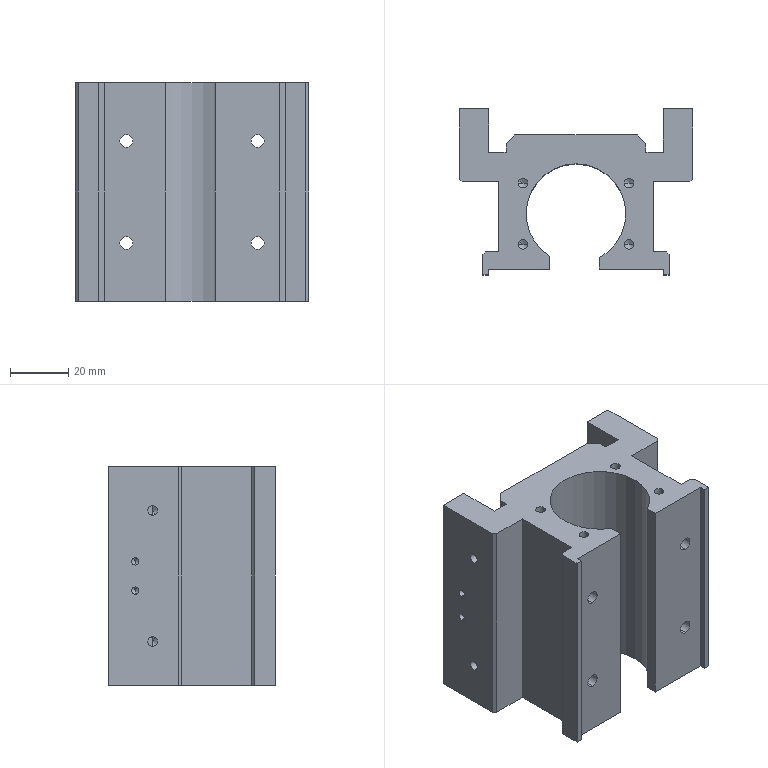Part | STEP file | 866-BDO024-93-04A | 1 solid | 134 faces | box 80 x 57 x 75 mm | volume 148857 mm3 | cylinder 56 | plane 50 | cone 28 | commonest cylinder face diameters 3.3 x16 2.5 x8 4.2 x8 4.5 x8 8 x8 5 x4